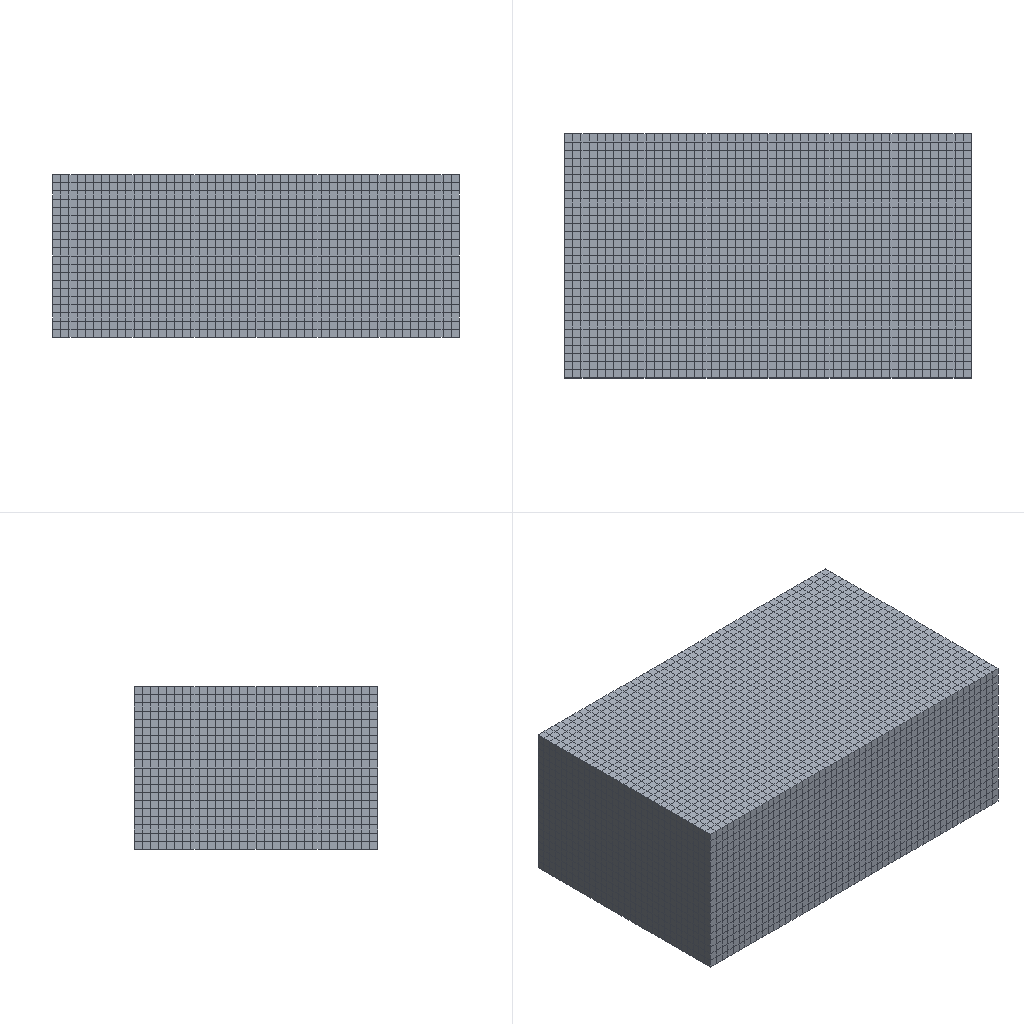Simulation study | abaqus
Set-up summary:
category,name,step,type,value,unit,region
solver,abaqus
solver,version,,,Abaqus/Explicit 2020
units,not stated in the deck,,not stated
analysis,deck,,transient,transient
load_step,Step-1,Step-1,transient
load_step,requested,,,1
mesh,nodes,,,40918
mesh,elements,,,38148
element_type,R3D3,,rigid,790
element_type,R3D4,,rigid,7358
element_type,C3D8R,,solid,30000
load,load commands in deck,,count,3
bc,support commands in deck,,count,19
material,MATERIAL-1,,in results
check,setup vs results,,match,"per instance, exact: element labels, types and connectivity; labels of the nodes the elements use; coordinates of those nodes at SINGLE_PRECISION in 5 of 5 instance(s)"
Abaqus input file, long lists of numbers shortened:
*Heading
** Job name: Job-1 Model name: Model-1
** Generated by: Abaqus/CAE 2020
*Preprint, echo=NO, model=NO, history=NO, contact=NO
**
** PARTS
**
*Part, name=P4-3
*Node
      1,  -324.87,         -15.,   68.03
      2,  -313.233,         -15.,    69.027
** (795 more lines like these left out)
*Element, type=R3D4
1,  1, 45, 54,  4
2, 45, 46, 53, 54
** (778 more lines like these left out)
*Element, type=R3D3
277, 177,  11, 178
278, 457, 429, 427
** (36 more lines like these left out)
*Node
    798,  -307.871,        -35.5,   72.748
*Nset, nset=P4-3-RefPt_, internal
798,
*Elset, elset=P4-3, generate
   1,  818,    1
*End Part
**
*Part, name=P4-4
*Node
      1,   -330.216,          15.,   67.573
      2,  -321.836,          15.,   68.29
** (849 more lines like these left out)
*Element, type=R3D4
1,  1, 51, 58,  4
2, 51, 52, 57, 58
** (828 more lines like these left out)
*Element, type=R3D3
309, 138,  24, 139
310,  34, 131, 562
** (44 more lines like these left out)
*Node
    852,  -307.871,         35.5,   72.748
*Nset, nset=P4-4-RefPt_, internal
852,
*Elset, elset=P4-4, generate
   1,  876,    1
*End Part
**
*Part, name=P4-5
*Node
      1,  -269.053,         -10.,   6.217
      2,    -273.038,         -10.,   5.876
** (2926 more lines like these left out)
*Element, type=R3D4
1,   1, 204, 209,   4
2, 204, 205, 208, 209
** (2784 more lines like these left out)
*Element, type=R3D3
344, 667, 127, 350
345, 667, 350, 130
** (334 more lines like these left out)
*Node
   2929,  -301.421, -2.84217094e-14,  -2.577
*Nset, nset=P4-5-RefPt_, internal
2929,
*Elset, elset=P4-5, generate
    1,  3122,     1
*End Part
**
*Part, name=Part-1
*Node
      1,  -277.257,        -10.5,   78.581
      2,  -277.257,        -14.5,   78.581
** (3135 more lines like these left out)
*Element, type=R3D4
 1,    1,  284, 1057,  292
 2,  284,  285, 1058, 1057
** (2960 more lines like these left out)
*Element, type=R3D3
585, 1176,  286,  285
591, 1179,  295,  294
** (368 more lines like these left out)
*Node
   3138,  -309.714, -6.39488462e-14,    94.269
*Nset, nset=Part-1-RefPt_, internal
3138,
*Elset, elset=Part-1, generate
    1,  3332,     1
*End Part
**
*Part, name=work
*Node
      1,           0.,         -30.,          20.
      2,           0.,         -29.,          20.
** (33199 more lines like these left out)
*Element, type=C3D8R
    1,   652,   653,   684,   683,     1,     2,    33,    32
    2,   653,   654,   685,   684,     2,     3,    34,    33
** (29998 more lines like these left out)
*Nset, nset=Set-1, generate
     1,  33201,      1
*Elset, elset=Set-1, generate
     1,  30000,      1
** Section: Section-1
*Solid Section, elset=Set-1, material=Material-1
,
*End Part
**
**
** ASSEMBLY
**
*Assembly, name=Assembly
**
*Instance, name=P4-3-1, part=P4-3
300.319,           0., -120.904
300.319,           0., -120.904, 300.319, 1., -120.904, 5.
*End Instance
**
*Instance, name=P4-4-1, part=P4-4
300.319,           0., -120.904
300.319,           0., -120.904, 300.319, 1., -120.904, 5.
*End Instance
**
*Instance, name=P4-5-1, part=P4-5
300.498,           0., -78.704
300.498,           0., -78.704, 300.498, 1., -78.704, 5.
*End Instance
**
*Instance, name=Part-1-1, part=Part-1
300.319,           0., -120.904
300.319,           0., -120.904, 300.319, 1., -120.904, 5.
*End Instance
**
*Instance, name=work-1, part=work
  -25.066,          15.,   -35.954
*End Instance
**
*Nset, nset=Set-1, instance=Part-1-1
 3138,
*Nset, nset=Set-2, instance=P4-4-1
 852,
*Nset, nset=Set-3, instance=P4-3-1
 798,
*Nset, nset=Set-4, instance=P4-5-1
 2929,
*Rigid Body, ref node=P4-3-1.P4-3-RefPt_, elset=P4-3-1.P4-3
*Rigid Body, ref node=P4-4-1.P4-4-RefPt_, elset=P4-4-1.P4-4
*Rigid Body, ref node=P4-5-1.P4-5-RefPt_, elset=P4-5-1.P4-5
*Rigid Body, ref node=Part-1-1.Part-1-RefPt_, elset=Part-1-1.Part-1
*End Assembly
**
** MATERIALS
**
*Material, name=Material-1
*Density
 2.7e-09,
*Elastic
69000., 0.29
*Plastic
500.,0.
**
** INTERACTION PROPERTIES
**
*Surface Interaction, name=IntProp-1
*Friction
 0.1,
*Surface Behavior, pressure-overclosure=HARD
** ----------------------------------------------------------------
**
** STEP: Step-1
**
*Step, name=Step-1, nlgeom=YES
*Dynamic, Explicit
, 0.1
*Bulk Viscosity
0.06, 1.2
** Mass Scaling: Semi-Automatic
**               Whole Model
*Fixed Mass Scaling, factor=5000.
**
** BOUNDARY CONDITIONS
**
** Name: BC-1 Type: 对称/反对称/完全固定
*Boundary
Set-1, ENCASTRE
** Name: [REDACTED] : Velocity/Angular velocity
*Boundary, type=VELOCITY
Set-2, 1, 1
Set-2, 2, 2, -40.
Set-2, 3, 3
Set-2, 4, 4
Set-2, 5, 5
Set-2, 6, 6
** Name: [REDACTED]
*Boundary, type=VELOCITY
Set-3, 1, 1
Set-3, 2, 2, 40.
Set-3, 3, 3
Set-3, 4, 4
Set-3, 5, 5
Set-3, 6, 6
** Name: [REDACTED] : Velocity/Angular velocity
*Boundary, type=VELOCITY
Set-4, 1, 1
Set-4, 2, 2
Set-4, 3, 3, 100.
Set-4, 4, 4
Set-4, 5, 5
Set-4, 6, 6
**
** INTERACTIONS
**
** Interaction: Int-1
*Contact, op=NEW
*Contact Inclusions, ALL EXTERIOR
*Contact Property Assignment
 ,  , IntProp-1
**
** OUTPUT REQUESTS
**
*Restart, write, number interval=1, time marks=NO
**
** FIELD OUTPUT: F-Output-1
**
*Output, field, number interval=50
*Node Output
A, CF, RF, RM, RT, U, V
*Element Output, directions=YES
E, EVF, LE, MISES, MISESMAX, PE, PEEQ, PEEQVAVG, PEVAVG, S, SEQUT, SVAVG, YIELDPOT
*Contact Output
CDISP, CSTRESS
**
** HISTORY OUTPUT: H-Output-1
**
*Output, history, variable=PRESELECT
*End Step
Results summary:
result,step,Step-1,completed,increments=29423 time=0.1/0.1
result,analysis,,,transient
result,last_loadstep,,,1
result,primary field,,,U
result,reaction total,,FX,1638.887,model units
result,reaction total,,FY,12666.074,model units
result,reaction total,,FZ,-2628.562,model units